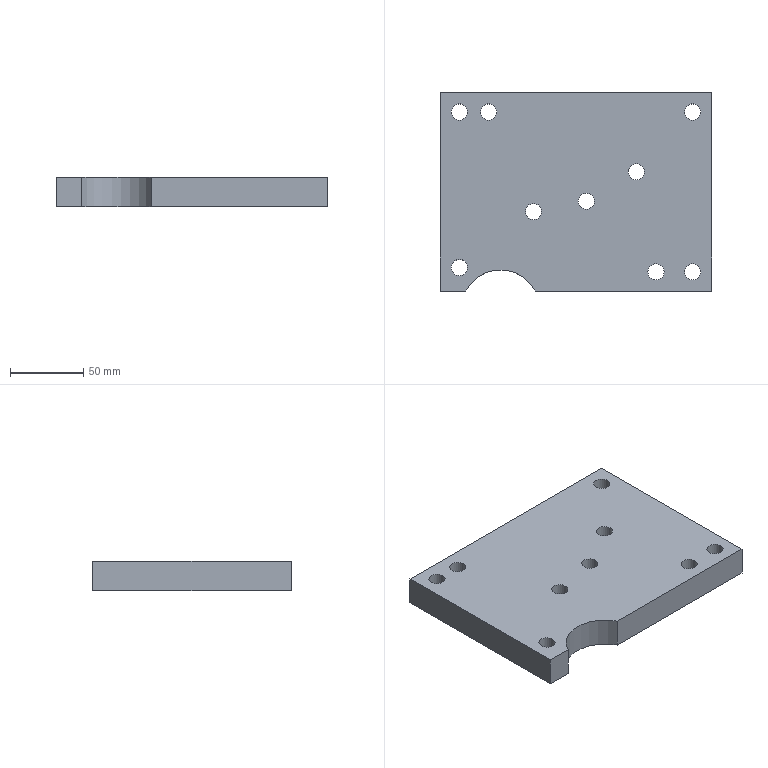Part | STEP file | 112_id2990_x_t | 1 solid | 17 faces | box 185 x 135 x 20 mm | volume 472603 mm3 | cylinder 10 | plane 7 | commonest cylinder face diameters 11 x9 53 x1